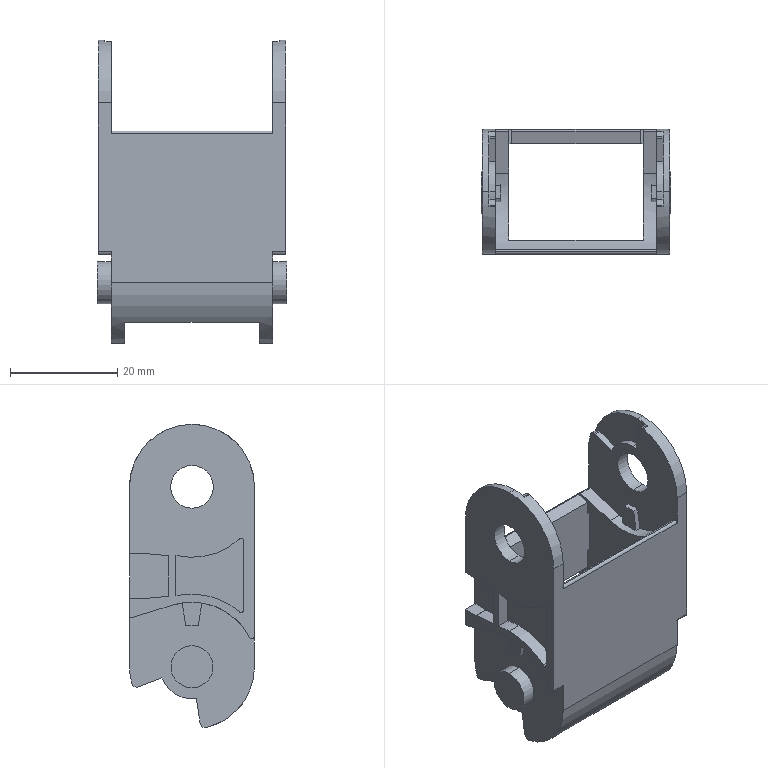Part | 1 solid | 142 faces | box 35.2 x 23.26 x 56.462 mm | volume 9320 mm3 | plane 80 | cylinder 62 | commonest cylinder face diameters 2 x12 1 x10 0.6 x8 23.26 x7 11.94 x6 24.06 x5